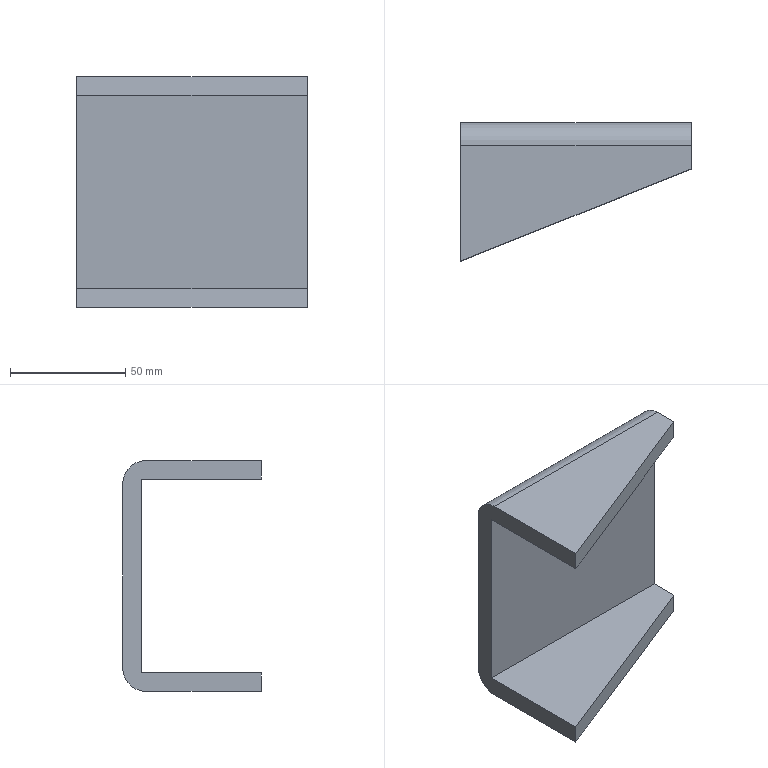Part | SolidWorks | features Fillet 2, Extrusion 1, Shell 1 | 1 solid | 12 faces | box 100 x 60 x 100 mm | volume 126908 mm3 | plane 10 | cylinder 2 | commonest cylinder face diameters 20 x2
STEP:
#1=CARTESIAN_POINT('',(100.,60.,10.));
#2=VERTEX_POINT('',#1);
#3=CARTESIAN_POINT('',(0.,60.,10.));
#4=VERTEX_POINT('',#3);
#5=CARTESIAN_POINT('',(0.,60.,10.));
#6=DIRECTION('',(-1.,0.,0.));
#7=VECTOR('',#6,1000.);
#8=LINE('',#5,#7);
#9=EDGE_CURVE('',#2,#4,#8,.T.);
#10=ORIENTED_EDGE('',*,*,#9,.F.);
#11=CARTESIAN_POINT('',(100.,50.,0.));
#12=VERTEX_POINT('',#11);
#13=CARTESIAN_POINT('',(100.,50.,10.));
#14=DIRECTION('',(1.,0.,0.));
#15=DIRECTION('',(0.,0.,1.));
#16=AXIS2_PLACEMENT_3D('',#13,#14,#15);
#17=CIRCLE('',#16,10.);
#18=EDGE_CURVE('',#12,#2,#17,.T.);
#19=ORIENTED_EDGE('',*,*,#18,.F.);
#20=CARTESIAN_POINT('',(0.,50.,0.));
#21=VERTEX_POINT('',#20);
#22=CARTESIAN_POINT('',(0.,50.,0.));
#23=DIRECTION('',(1.,0.,0.));
#24=VECTOR('',#23,1000.);
#25=LINE('',#22,#24);
#26=EDGE_CURVE('',#21,#12,#25,.T.);
#27=ORIENTED_EDGE('',*,*,#26,.F.);
#28=CARTESIAN_POINT('',(0.,50.,10.));
#29=DIRECTION('',(-1.,0.,0.));
#30=DIRECTION('',(0.,0.,-1.));
#31=AXIS2_PLACEMENT_3D('',#28,#29,#30);
#32=CIRCLE('',#31,10.);
#33=EDGE_CURVE('',#4,#21,#32,.T.);
#34=ORIENTED_EDGE('',*,*,#33,.F.);
#35=EDGE_LOOP('',(#10,#19,#27,#34));
#36=FACE_OUTER_BOUND('',#35,.T.);
#37=CARTESIAN_POINT('',(0.,50.,10.));
#38=DIRECTION('',(1.,0.,0.));
#39=DIRECTION('',(0.,0.,-1.));
#40=AXIS2_PLACEMENT_3D('',#37,#38,#39);
#41=CYLINDRICAL_SURFACE('',#40,10.);
#42=ADVANCED_FACE('',(#36),#41,.T.);
#43=CARTESIAN_POINT('',(100.,50.,100.));
#44=VERTEX_POINT('',#43);
#45=CARTESIAN_POINT('',(0.,50.,100.));
#46=VERTEX_POINT('',#45);
#47=CARTESIAN_POINT('',(0.,50.,100.));
#48=DIRECTION('',(-1.,0.,0.));
#49=VECTOR('',#48,1000.);
#50=LINE('',#47,#49);
#51=EDGE_CURVE('',#44,#46,#50,.T.);
#52=ORIENTED_EDGE('',*,*,#51,.F.);
#53=CARTESIAN_POINT('',(100.,60.,90.));
#54=VERTEX_POINT('',#53);
#55=CARTESIAN_POINT('',(100.,50.,90.));
#56=DIRECTION('',(1.,0.,0.));
#57=DIRECTION('',(0.,0.,1.));
#58=AXIS2_PLACEMENT_3D('',#55,#56,#57);
#59=CIRCLE('',#58,10.);
#60=EDGE_CURVE('',#54,#44,#59,.T.);
#61=ORIENTED_EDGE('',*,*,#60,.F.);
#62=CARTESIAN_POINT('',(0.,60.,90.));
#63=VERTEX_POINT('',#62);
#64=CARTESIAN_POINT('',(0.,60.,90.));
#65=DIRECTION('',(1.,0.,0.));
#66=VECTOR('',#65,1000.);
#67=LINE('',#64,#66);
#68=EDGE_CURVE('',#63,#54,#67,.T.);
#69=ORIENTED_EDGE('',*,*,#68,.F.);
#70=CARTESIAN_POINT('',(0.,50.,90.));
#71=DIRECTION('',(-1.,0.,0.));
#72=DIRECTION('',(0.,0.,-1.));
#73=AXIS2_PLACEMENT_3D('',#70,#71,#72);
#74=CIRCLE('',#73,10.);
#75=EDGE_CURVE('',#46,#63,#74,.T.);
#76=ORIENTED_EDGE('',*,*,#75,.F.);
#77=EDGE_LOOP('',(#52,#61,#69,#76));
#78=FACE_OUTER_BOUND('',#77,.T.);
#79=CARTESIAN_POINT('',(0.,50.,90.));
#80=DIRECTION('',(-1.,0.,0.));
#81=DIRECTION('',(0.,0.,1.));
#82=AXIS2_PLACEMENT_3D('',#79,#80,#81);
#83=CYLINDRICAL_SURFACE('',#82,10.);
#84=ADVANCED_FACE('',(#78),#83,.T.);
#85=CARTESIAN_POINT('',(0.,0.,8.));
#86=VERTEX_POINT('',#85);
#87=CARTESIAN_POINT('',(100.,40.,8.));
#88=VERTEX_POINT('',#87);
#89=CARTESIAN_POINT('',(0.,0.,8.));
#90=DIRECTION('',(0.9285,0.3714,0.));
#91=VECTOR('',#90,1000.);
#92=LINE('',#89,#91);
#93=EDGE_CURVE('',#86,#88,#92,.T.);
#94=ORIENTED_EDGE('',*,*,#93,.F.);
#95=CARTESIAN_POINT('',(0.,0.,0.));
#96=VERTEX_POINT('',#95);
#97=CARTESIAN_POINT('',(0.,0.,100.));
#98=DIRECTION('',(0.,0.,-1.));
#99=VECTOR('',#98,1000.);
#100=LINE('',#97,#99);
#101=EDGE_CURVE('',#86,#96,#100,.T.);
#102=ORIENTED_EDGE('',*,*,#101,.T.);
#103=CARTESIAN_POINT('',(100.,40.,0.));
#104=VERTEX_POINT('',#103);
#105=CARTESIAN_POINT('',(100.,40.,0.));
#106=DIRECTION('',(0.9285,0.3714,0.));
#107=VECTOR('',#106,1000.);
#108=LINE('',#105,#107);
#109=EDGE_CURVE('',#96,#104,#108,.T.);
#110=ORIENTED_EDGE('',*,*,#109,.T.);
#111=CARTESIAN_POINT('',(100.,40.,100.));
#112=DIRECTION('',(0.,0.,-1.));
#113=VECTOR('',#112,1000.);
#114=LINE('',#111,#113);
#115=EDGE_CURVE('',#88,#104,#114,.T.);
#116=ORIENTED_EDGE('',*,*,#115,.F.);
#117=EDGE_LOOP('',(#94,#102,#110,#116));
#118=FACE_OUTER_BOUND('',#117,.T.);
#119=CARTESIAN_POINT('',(100.,40.,100.));
#120=DIRECTION('',(-0.3714,0.9285,0.));
#121=DIRECTION('',(-0.9285,-0.3714,0.));
#122=AXIS2_PLACEMENT_3D('',#119,#120,#121);
#123=PLANE('',#122);
#124=ADVANCED_FACE('',(#118),#123,.F.);
#125=CARTESIAN_POINT('',(100.,60.,0.));
#126=DIRECTION('',(0.,1.,0.));
#127=VECTOR('',#126,1000.);
#128=LINE('',#125,#127);
#129=EDGE_CURVE('',#104,#12,#128,.T.);
#130=ORIENTED_EDGE('',*,*,#129,.T.);
#131=ORIENTED_EDGE('',*,*,#18,.T.);
#132=CARTESIAN_POINT('',(100.,60.,100.));
#133=DIRECTION('',(0.,0.,-1.));
#134=VECTOR('',#133,1000.);
#135=LINE('',#132,#134);
#136=EDGE_CURVE('',#54,#2,#135,.T.);
#137=ORIENTED_EDGE('',*,*,#136,.F.);
#138=ORIENTED_EDGE('',*,*,#60,.T.);
#139=CARTESIAN_POINT('',(100.,40.,100.));
#140=VERTEX_POINT('',#139);
#141=CARTESIAN_POINT('',(100.,60.,100.));
#142=DIRECTION('',(0.,1.,0.));
#143=VECTOR('',#142,1000.);
#144=LINE('',#141,#143);
#145=EDGE_CURVE('',#140,#44,#144,.T.);
#146=ORIENTED_EDGE('',*,*,#145,.F.);
#147=CARTESIAN_POINT('',(100.,40.,92.));
#148=VERTEX_POINT('',#147);
#149=CARTESIAN_POINT('',(100.,40.,100.));
#150=DIRECTION('',(0.,0.,-1.));
#151=VECTOR('',#150,1000.);
#152=LINE('',#149,#151);
#153=EDGE_CURVE('',#140,#148,#152,.T.);
#154=ORIENTED_EDGE('',*,*,#153,.T.);
#155=CARTESIAN_POINT('',(100.,52.,92.));
#156=VERTEX_POINT('',#155);
#157=CARTESIAN_POINT('',(100.,0.,92.));
#158=DIRECTION('',(0.,1.,0.));
#159=VECTOR('',#158,1000.);
#160=LINE('',#157,#159);
#161=EDGE_CURVE('',#148,#156,#160,.T.);
#162=ORIENTED_EDGE('',*,*,#161,.T.);
#163=CARTESIAN_POINT('',(100.,52.,8.));
#164=VERTEX_POINT('',#163);
#165=CARTESIAN_POINT('',(100.,52.,100.));
#166=DIRECTION('',(0.,0.,-1.));
#167=VECTOR('',#166,1000.);
#168=LINE('',#165,#167);
#169=EDGE_CURVE('',#156,#164,#168,.T.);
#170=ORIENTED_EDGE('',*,*,#169,.T.);
#171=CARTESIAN_POINT('',(100.,0.,8.));
#172=DIRECTION('',(0.,1.,0.));
#173=VECTOR('',#172,1000.);
#174=LINE('',#171,#173);
#175=EDGE_CURVE('',#88,#164,#174,.T.);
#176=ORIENTED_EDGE('',*,*,#175,.F.);
#177=ORIENTED_EDGE('',*,*,#115,.T.);
#178=EDGE_LOOP('',(#130,#131,#137,#138,#146,#154,#162,#170,#176,#177));
#179=FACE_OUTER_BOUND('',#178,.T.);
#180=CARTESIAN_POINT('',(100.,60.,100.));
#181=DIRECTION('',(-1.,0.,0.));
#182=DIRECTION('',(0.,0.,1.));
#183=AXIS2_PLACEMENT_3D('',#180,#181,#182);
#184=PLANE('',#183);
#185=ADVANCED_FACE('',(#179),#184,.F.);
#186=CARTESIAN_POINT('',(0.,60.,100.));
#187=DIRECTION('',(0.,0.,-1.));
#188=VECTOR('',#187,1000.);
#189=LINE('',#186,#188);
#190=EDGE_CURVE('',#63,#4,#189,.T.);
#191=ORIENTED_EDGE('',*,*,#190,.T.);
#192=ORIENTED_EDGE('',*,*,#33,.T.);
#193=CARTESIAN_POINT('',(0.,0.,0.));
#194=DIRECTION('',(0.,-1.,0.));
#195=VECTOR('',#194,1000.);
#196=LINE('',#193,#195);
#197=EDGE_CURVE('',#21,#96,#196,.T.);
#198=ORIENTED_EDGE('',*,*,#197,.T.);
#199=ORIENTED_EDGE('',*,*,#101,.F.);
#200=CARTESIAN_POINT('',(0.,52.,8.));
#201=VERTEX_POINT('',#200);
#202=CARTESIAN_POINT('',(0.,0.,8.));
#203=DIRECTION('',(0.,-1.,0.));
#204=VECTOR('',#203,1000.);
#205=LINE('',#202,#204);
#206=EDGE_CURVE('',#201,#86,#205,.T.);
#207=ORIENTED_EDGE('',*,*,#206,.F.);
#208=CARTESIAN_POINT('',(0.,52.,92.));
#209=VERTEX_POINT('',#208);
#210=CARTESIAN_POINT('',(0.,52.,100.));
#211=DIRECTION('',(0.,0.,-1.));
#212=VECTOR('',#211,1000.);
#213=LINE('',#210,#212);
#214=EDGE_CURVE('',#209,#201,#213,.T.);
#215=ORIENTED_EDGE('',*,*,#214,.F.);
#216=CARTESIAN_POINT('',(0.,0.,92.));
#217=VERTEX_POINT('',#216);
#218=CARTESIAN_POINT('',(0.,0.,92.));
#219=DIRECTION('',(0.,-1.,0.));
#220=VECTOR('',#219,1000.);
#221=LINE('',#218,#220);
#222=EDGE_CURVE('',#209,#217,#221,.T.);
#223=ORIENTED_EDGE('',*,*,#222,.T.);
#224=CARTESIAN_POINT('',(0.,0.,100.));
#225=VERTEX_POINT('',#224);
#226=CARTESIAN_POINT('',(0.,0.,100.));
#227=DIRECTION('',(0.,0.,-1.));
#228=VECTOR('',#227,1000.);
#229=LINE('',#226,#228);
#230=EDGE_CURVE('',#225,#217,#229,.T.);
#231=ORIENTED_EDGE('',*,*,#230,.F.);
#232=CARTESIAN_POINT('',(0.,0.,100.));
#233=DIRECTION('',(0.,-1.,0.));
#234=VECTOR('',#233,1000.);
#235=LINE('',#232,#234);
#236=EDGE_CURVE('',#46,#225,#235,.T.);
#237=ORIENTED_EDGE('',*,*,#236,.F.);
#238=ORIENTED_EDGE('',*,*,#75,.T.);
#239=EDGE_LOOP('',(#191,#192,#198,#199,#207,#215,#223,#231,#237,#238));
#240=FACE_OUTER_BOUND('',#239,.T.);
#241=CARTESIAN_POINT('',(0.,0.,100.));
#242=DIRECTION('',(1.,0.,0.));
#243=DIRECTION('',(0.,0.,-1.));
#244=AXIS2_PLACEMENT_3D('',#241,#242,#243);
#245=PLANE('',#244);
#246=ADVANCED_FACE('',(#240),#245,.F.);
#247=ORIENTED_EDGE('',*,*,#230,.T.);
#248=CARTESIAN_POINT('',(0.,0.,92.));
#249=DIRECTION('',(0.9285,0.3714,0.));
#250=VECTOR('',#249,1000.);
#251=LINE('',#248,#250);
#252=EDGE_CURVE('',#217,#148,#251,.T.);
#253=ORIENTED_EDGE('',*,*,#252,.T.);
#254=ORIENTED_EDGE('',*,*,#153,.F.);
#255=CARTESIAN_POINT('',(100.,40.,100.));
#256=DIRECTION('',(0.9285,0.3714,0.));
#257=VECTOR('',#256,1000.);
#258=LINE('',#255,#257);
#259=EDGE_CURVE('',#225,#140,#258,.T.);
#260=ORIENTED_EDGE('',*,*,#259,.F.);
#261=EDGE_LOOP('',(#247,#253,#254,#260));
#262=FACE_OUTER_BOUND('',#261,.T.);
#263=CARTESIAN_POINT('',(100.,40.,100.));
#264=DIRECTION('',(-0.3714,0.9285,0.));
#265=DIRECTION('',(-0.9285,-0.3714,0.));
#266=AXIS2_PLACEMENT_3D('',#263,#264,#265);
#267=PLANE('',#266);
#268=ADVANCED_FACE('',(#262),#267,.F.);
#269=ORIENTED_EDGE('',*,*,#136,.T.);
#270=ORIENTED_EDGE('',*,*,#9,.T.);
#271=ORIENTED_EDGE('',*,*,#190,.F.);
#272=ORIENTED_EDGE('',*,*,#68,.T.);
#273=EDGE_LOOP('',(#269,#270,#271,#272));
#274=FACE_OUTER_BOUND('',#273,.T.);
#275=CARTESIAN_POINT('',(0.,60.,100.));
#276=DIRECTION('',(0.,-1.,0.));
#277=DIRECTION('',(0.,0.,-1.));
#278=AXIS2_PLACEMENT_3D('',#275,#276,#277);
#279=PLANE('',#278);
#280=ADVANCED_FACE('',(#274),#279,.F.);
#281=ORIENTED_EDGE('',*,*,#145,.T.);
#282=ORIENTED_EDGE('',*,*,#51,.T.);
#283=ORIENTED_EDGE('',*,*,#236,.T.);
#284=ORIENTED_EDGE('',*,*,#259,.T.);
#285=EDGE_LOOP('',(#281,#282,#283,#284));
#286=FACE_OUTER_BOUND('',#285,.T.);
#287=CARTESIAN_POINT('',(0.,0.,100.));
#288=DIRECTION('',(0.,0.,-1.));
#289=DIRECTION('',(-1.,0.,0.));
#290=AXIS2_PLACEMENT_3D('',#287,#288,#289);
#291=PLANE('',#290);
#292=ADVANCED_FACE('',(#286),#291,.F.);
#293=ORIENTED_EDGE('',*,*,#197,.F.);
#294=ORIENTED_EDGE('',*,*,#26,.T.);
#295=ORIENTED_EDGE('',*,*,#129,.F.);
#296=ORIENTED_EDGE('',*,*,#109,.F.);
#297=EDGE_LOOP('',(#293,#294,#295,#296));
#298=FACE_OUTER_BOUND('',#297,.T.);
#299=CARTESIAN_POINT('',(0.,0.,0.));
#300=DIRECTION('',(0.,0.,-1.));
#301=DIRECTION('',(-1.,0.,0.));
#302=AXIS2_PLACEMENT_3D('',#299,#300,#301);
#303=PLANE('',#302);
#304=ADVANCED_FACE('',(#298),#303,.T.);
#305=CARTESIAN_POINT('',(0.,52.,8.));
#306=DIRECTION('',(-1.,0.,0.));
#307=VECTOR('',#306,1000.);
#308=LINE('',#305,#307);
#309=EDGE_CURVE('',#164,#201,#308,.T.);
#310=ORIENTED_EDGE('',*,*,#309,.F.);
#311=ORIENTED_EDGE('',*,*,#169,.F.);
#312=CARTESIAN_POINT('',(0.,52.,92.));
#313=DIRECTION('',(-1.,0.,0.));
#314=VECTOR('',#313,1000.);
#315=LINE('',#312,#314);
#316=EDGE_CURVE('',#156,#209,#315,.T.);
#317=ORIENTED_EDGE('',*,*,#316,.T.);
#318=ORIENTED_EDGE('',*,*,#214,.T.);
#319=EDGE_LOOP('',(#310,#311,#317,#318));
#320=FACE_OUTER_BOUND('',#319,.T.);
#321=CARTESIAN_POINT('',(0.,52.,100.));
#322=DIRECTION('',(0.,-1.,0.));
#323=DIRECTION('',(0.,0.,-1.));
#324=AXIS2_PLACEMENT_3D('',#321,#322,#323);
#325=PLANE('',#324);
#326=ADVANCED_FACE('',(#320),#325,.T.);
#327=ORIENTED_EDGE('',*,*,#252,.F.);
#328=ORIENTED_EDGE('',*,*,#222,.F.);
#329=ORIENTED_EDGE('',*,*,#316,.F.);
#330=ORIENTED_EDGE('',*,*,#161,.F.);
#331=EDGE_LOOP('',(#327,#328,#329,#330));
#332=FACE_OUTER_BOUND('',#331,.T.);
#333=CARTESIAN_POINT('',(0.,0.,92.));
#334=DIRECTION('',(0.,0.,-1.));
#335=DIRECTION('',(-1.,0.,0.));
#336=AXIS2_PLACEMENT_3D('',#333,#334,#335);
#337=PLANE('',#336);
#338=ADVANCED_FACE('',(#332),#337,.T.);
#339=ORIENTED_EDGE('',*,*,#93,.T.);
#340=ORIENTED_EDGE('',*,*,#175,.T.);
#341=ORIENTED_EDGE('',*,*,#309,.T.);
#342=ORIENTED_EDGE('',*,*,#206,.T.);
#343=EDGE_LOOP('',(#339,#340,#341,#342));
#344=FACE_OUTER_BOUND('',#343,.T.);
#345=CARTESIAN_POINT('',(0.,0.,8.));
#346=DIRECTION('',(0.,0.,-1.));
#347=DIRECTION('',(-1.,0.,0.));
#348=AXIS2_PLACEMENT_3D('',#345,#346,#347);
#349=PLANE('',#348);
#350=ADVANCED_FACE('',(#344),#349,.F.);
#351=CLOSED_SHELL('',(#42,#84,#124,#185,#246,#268,#280,#292,#304,#326,#338,#350));
#352=MANIFOLD_SOLID_BREP('',#351);
#353=CARTESIAN_POINT('',(0.,0.,0.));
#354=DIRECTION('',(0.,0.,1.));
#355=DIRECTION('',(1.,0.,0.));
#356=AXIS2_PLACEMENT_3D('',#353,#354,#355);
#357=(LENGTH_UNIT()NAMED_UNIT(*)SI_UNIT(.MILLI.,.METRE.));
#358=UNCERTAINTY_MEASURE_WITH_UNIT(LENGTH_MEASURE(0.00001),#357,'','');
#359=(NAMED_UNIT(*)PLANE_ANGLE_UNIT()SI_UNIT($,.RADIAN.));
#360=(NAMED_UNIT(*)SI_UNIT($,.STERADIAN.)SOLID_ANGLE_UNIT());
#361=(GEOMETRIC_REPRESENTATION_CONTEXT(3)GLOBAL_UNCERTAINTY_ASSIGNED_CONTEXT((#358))GLOBAL_UNIT_ASSIGNED_CONTEXT((#357,#359,#360))REPRESENTATION_CONTEXT('',''));
#362=ADVANCED_BREP_SHAPE_REPRESENTATION('',(#352,#356),#361);